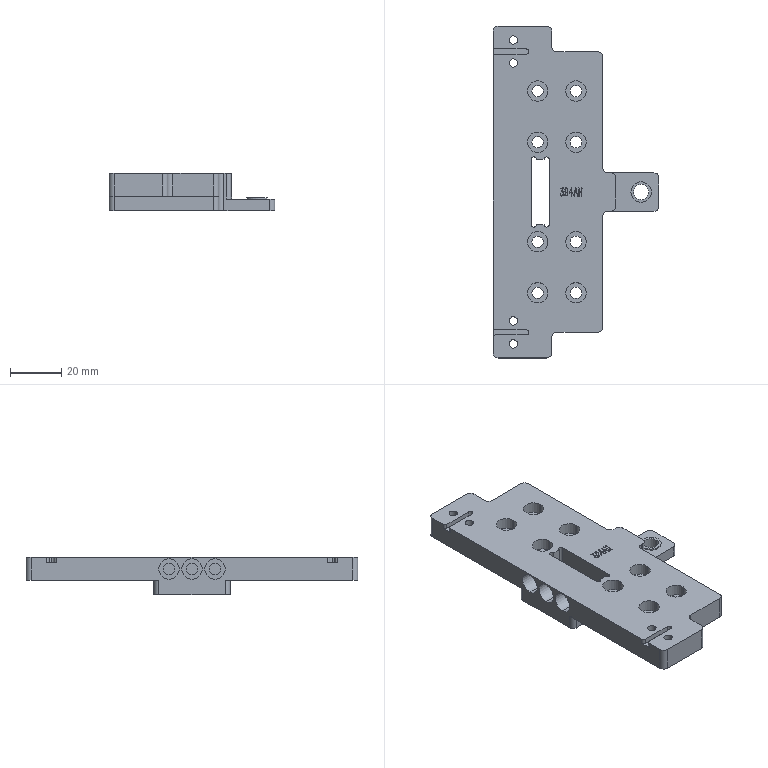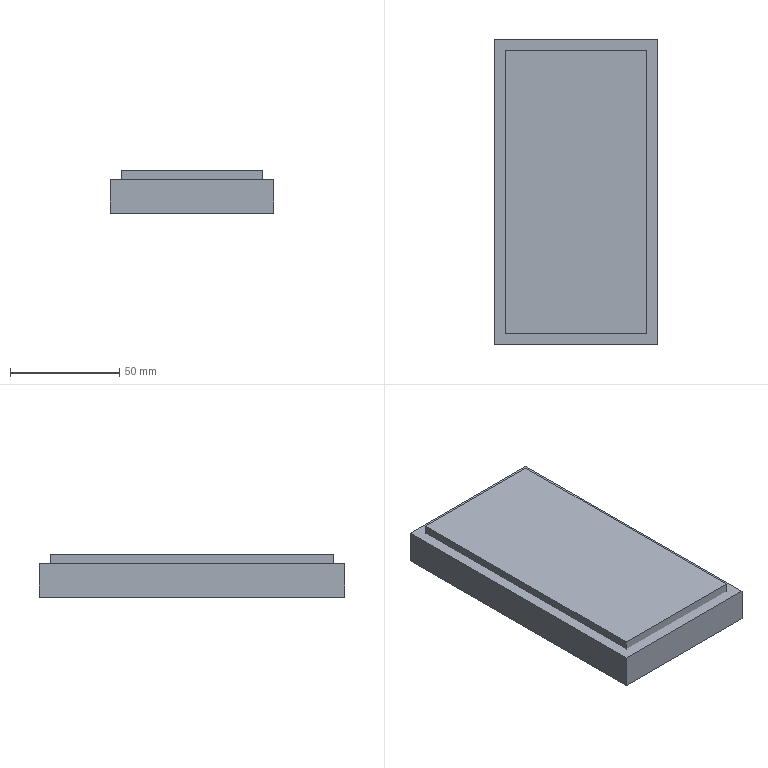CAM job | NX | 3+2 milling, drilling | part box 65 x 130 x 14.5 mm | stock box 75 x 140 x 19.5 mm
Tools:
number,name,description,diameter,corner_radius,flute_length,length,flutes
19,D80,Milling Tool-5 Parameters,80.0,0.0,50.0,75.0,2
1,D6A45,Milling Tool-5 Parameters,6.0,0.0,50.0,75.0,2
3,3.3ZT,Drilling Tool,3.3,0.0,35.0,50.0,2
2,2.0ZT,Drilling Tool,2.0,0.0,35.0,50.0,2
8,4.5ZT,Drilling Tool,4.5,0.0,35.0,50.0,2
15,D10,Milling Tool-5 Parameters,10.0,0.0,50.0,75.0,2
14,D10JING,Milling Tool-5 Parameters,10.0,0.0,50.0,75.0,2
11,D4,Milling Tool-5 Parameters,4.0,0.0,50.0,75.0,2
16,D3,Milling Tool-5 Parameters,3.0,0.0,50.0,75.0,2
17,D1.5,Milling Tool-5 Parameters,1.5,0.0,50.0,75.0,2
20,D2,Milling Tool-5 Parameters,2.0,0.0,50.0,75.0,2
12,D6,Milling Tool-5 Parameters,6.0,0.0,50.0,75.0,2
Operations:
program,operation,operation_type,tool,method,geometry_group,spindle_rpm,surface_speed,feed_per_tooth,feed_cut,feed_plunge,cut_length_mm,path_length_mm,cut_time_min,machine_time_min
1,FLOOR_WALL_COPY,VolumeBased25DMillingOperation,D80,METHOD,A,6500.0,1633.0,0.1154,1500.0,100.0,236.0,290.0,0.1573,0.1627
1,DRILLING_COPY_1,Operation,D6A45,METHOD,A,5000.0,94.0,0.035,350.0,0.0,64.0,435.704,0.1829,0.22
1,DRILLING_COPY_1_COPY_1,Operation,D6A45,METHOD,A,5000.0,94.0,0.035,350.0,0.0,20.4,229.818,0.0583,0.0792
1,DRILLING_COPY_COPY,Operation,3.3ZT,METHOD,A,2000.0,20.0,0.045,180.0,0.0,57.966,304.95,0.322,0.3467
1,DRILLING_COPY_COPY_COPY_2,Operation,4.5ZT,METHOD,A,2000.0,20.0,0.045,180.0,0.0,98.816,518.224,0.549,0.5909
1,DRILLING_COPY_COPY_COPY_2_COPY,Operation,4.5ZT,METHOD,A,2000.0,20.0,0.045,180.0,0.0,19.852,99.704,0.1103,0.1183
1,DRILLING_COPY_COPY_COPY_1,Operation,2.0ZT,METHOD,A,3000.0,18.0,0.02,120.0,0.0,76.403,259.145,0.6367,0.655
1,ADAPTIVE_MILLING,CavityMilling,D10,METHOD,A,9500.0,298.0,0.1579,3000.0,1000.0,8643.682,8726.682,2.883,2.892
1,CAVITY_MILL,CavityMilling,D10,METHOD,A,9500.0,298.0,0.1316,2500.0,700.0,1723.228,1807.474,0.8227,0.8311
1,ZLEVEL_PROFILE_COPY_1_COPY_COPY_1,ZLevelMilling,D10JING,METHOD,A,9500.0,298.0,0.0632,1200.0,1000.0,413.348,500.348,0.3451,0.3538
1,FLOOR_WALL,VolumeBased25DMillingOperation,D4,METHOD,A,9500.0,119.0,0.0658,1250.0,100.0,308.35,843.402,0.2467,0.3002
1,HOLE_MILLING,CylinderMilling,D4,METHOD,A,9500.0,119.0,0.0658,1250.0,100.0,86.431,169.931,0.0691,0.0775
1,HOLE_MILLING_COPY,CylinderMilling,D4,METHOD,A,9500.0,119.0,0.0658,1250.0,100.0,1433.215,2085.015,1.147,1.212
1,ZLEVEL_PROFILE,ZLevelMilling,D4,METHOD,A,9500.0,119.0,0.0947,1800.0,1000.0,1843.473,1914.973,1.04,1.047
1,ZLEVEL_PROFILE_COPY,ZLevelMilling,D4,METHOD,A,9500.0,119.0,0.0947,1800.0,1000.0,1222.518,2359.117,0.7522,0.8658
1,ZLEVEL_PROFILE_COPY_COPY,ZLevelMilling,D3,METHOD,A,9500.0,89.0,0.0632,1200.0,1000.0,1021.418,1667.76,0.8918,0.9564
1,PLANAR_MILL,PlanarMilling,D2,METHOD,A,9500.0,59.0,0.0579,1100.0,100.0,2792.659,4368.829,2.539,2.696
1,ZLEVEL_PROFILE_COPY_COPY_COPY,ZLevelMilling,D1.5,METHOD,A,9500.0,89.0,0.0632,1200.0,1000.0,1167.507,1488.16,0.9756,1.008
1,PLANAR_MILL_COPY_COPY_COPY_COPY_COPY_COPY_1,PlanarMilling,D6A45,METHOD,A,9500.0,179.0,0.0658,1250.0,100.0,741.251,1791.336,0.593,0.698
1,PLANAR_MILL_COPY_COPY_COPY_COPY_COPY_COPY_1_COPY_1,PlanarMilling,D6A45,METHOD,A,9500.0,179.0,0.0658,1250.0,100.0,20.128,98.128,0.0161,0.0239
1,PLANAR_MILL_COPY_COPY_COPY_COPY_COPY_COPY_1_COPY_1_COPY,PlanarMilling,D6A45,METHOD,A,9500.0,179.0,0.0658,1250.0,100.0,51.222,130.222,0.041,0.0489
1,TOOLCOMP11,CylinderMilling,D4,METHOD,A,9500.0,119.0,0.0658,1250.0,100.0,26.286,109.786,0.021,0.0294
1,TOOLCOMP11_COPY,CylinderMilling,D4,METHOD,A,9500.0,119.0,0.0658,1250.0,100.0,26.544,110.044,0.0212,0.0296
1,TOOLCOMP3,ZLevelMilling,D3,METHOD,A,9500.0,119.0,0.0632,1200.0,1000.0,173.258,403.087,0.1456,0.1686
1,TOOLCOMP3_COPY,ZLevelMilling,D3,METHOD,A,9500.0,119.0,0.0632,1200.0,1000.0,173.258,403.087,0.1456,0.1686
1,TOOLCOMP17,ZLevelMilling,D1.5,METHOD,A,9500.0,89.0,0.0632,1200.0,1000.0,66.164,295.844,0.0556,0.0786
2,ZLEVEL_PROFILE_1,ZLevelMilling,D10,METHOD,B,9500.0,298.0,0.1316,2500.0,1000.0,1531.3,2567.374,0.6216,0.7252
2,FLOOR_WALL_COPY_COPY,VolumeBased25DMillingOperation,D80,METHOD,B,6500.0,1633.0,0.1154,1500.0,100.0,1130.0,2258.801,0.7533,0.8662
2,FLOOR_WALL_COPY_COPY_COPY,VolumeBased25DMillingOperation,D80,METHOD,B,6500.0,1633.0,0.1154,1500.0,100.0,226.0,280.0,0.1507,0.1561
2,CAVITY_MILL_COPY_1,CavityMilling,D10,METHOD,B,9500.0,298.0,0.1316,2500.0,700.0,6050.283,6561.099,2.553,2.634
2,CAVITY_MILL_COPY_1_COPY,CavityMilling,D4,METHOD,B,9500.0,119.0,0.0868,1650.0,700.0,296.27,1038.574,0.2347,0.3089
2,FLOOR_WALL_COPY_1,VolumeBased25DMillingOperation,D4,METHOD,B,9500.0,119.0,0.0658,1250.0,100.0,1779.18,2143.577,1.423,1.46
2,FLOOR_WALL_COPY_1_COPY,VolumeBased25DMillingOperation,D4,METHOD,B,9500.0,119.0,0.0658,1250.0,100.0,1314.272,1707.962,1.051,1.091
2,ZLEVEL_PROFILE_COPY_COPY_COPY_1,ZLevelMilling,D3,METHOD,B,9500.0,89.0,0.0632,1200.0,1000.0,1356.7,2108.39,1.185,1.26
2,PLANAR_MILL_COPY,PlanarMilling,D2,METHOD,B,9500.0,59.0,0.0579,1100.0,100.0,3594.594,5393.105,3.268,3.448
2,CAVITY_MILL_COPY_1_COPY_COPY,CavityMilling,D2,METHOD,B,9500.0,59.0,0.0579,1100.0,700.0,454.157,2383.062,0.481,0.6738
2,PLANAR_MILL_COPY_COPY_COPY_COPY_COPY_COPY_1_COPY,PlanarMilling,D6A45,METHOD,B,9500.0,179.0,0.0658,1250.0,100.0,286.095,521.789,0.2289,0.2524
2,PLANAR_MILL_COPY_COPY_COPY_COPY_COPY_COPY_1_COPY_COPY,PlanarMilling,D6A45,METHOD,B,9500.0,179.0,0.0658,1250.0,100.0,416.792,961.146,0.3334,0.3879
2,PLANAR_MILL_COPY_COPY_COPY_COPY_COPY_COPY_1_COPY_COPY_COPY,PlanarMilling,D6A45,METHOD,B,9500.0,179.0,0.0658,1250.0,100.0,166.389,1124.005,0.1331,0.2289
2,DRILLING_COPY_1_COPY_1_COPY,Operation,D6A45,METHOD,B,5000.0,94.0,0.035,350.0,0.0,20.4,240.818,0.0583,0.0803
2,TOOLCOMP3_COPY_1,ZLevelMilling,D3,METHOD,B,9500.0,119.0,0.0632,1200.0,1000.0,346.513,792.086,0.2912,0.3357
2,TOOLCOMP111,VolumeBased25DMillingOperation,D4,METHOD,B,9500.0,119.0,0.0658,1250.0,100.0,228.782,453.494,0.183,0.2055
3,DRILLING_COPY_1_COPY,Operation,D6A45,METHOD,C,5000.0,94.0,0.035,350.0,0.0,12.0,108.974,0.0343,0.044
3,DRILLING_COPY_1_COPY_COPY,Operation,4.5ZT,METHOD,C,2000.0,28.0,0.05,200.0,0.0,62.556,210.085,0.3128,0.3275
3,HOLE_MILLING_1,CylinderMilling,D6,METHOD,C,9500.0,179.0,0.0737,1400.0,100.0,368.639,590.639,0.2633,0.2855
3,PLANAR_MILL_COPY_COPY_COPY_COPY_COPY_COPY_1_COPY_COPY_1,PlanarMilling,D6A45,METHOD,C,9500.0,179.0,0.0658,1250.0,100.0,78.759,271.358,0.063,0.0823